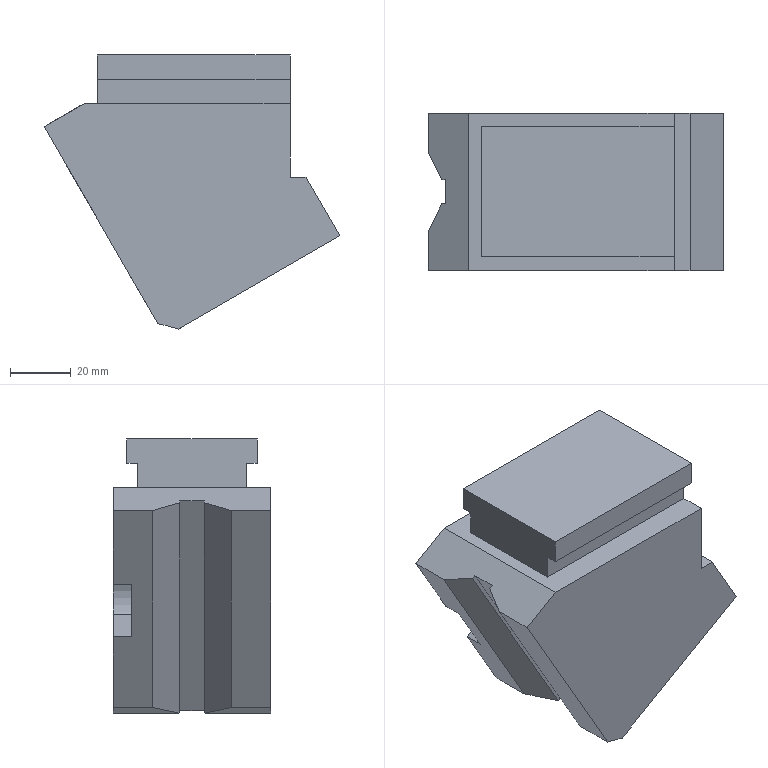Part | NX | features solid 2 | 1 solid | 33 faces | box 97.591 x 52 x 90.41 mm | volume 261017 mm3 | plane 31 | cylinder 2 | commonest cylinder face diameters 20 x2
STEP:
#1=CARTESIAN_POINT('',(-286.306,-188.,119.72));
#2=VERTEX_POINT('',#1);
#3=CARTESIAN_POINT('',(-339.567,-188.,88.97));
#4=VERTEX_POINT('',#3);
#5=CARTESIAN_POINT('',(-286.306,-188.,119.72));
#6=DIRECTION('',(-0.866,0.,-0.5));
#7=VECTOR('',#6,1000.);
#8=LINE('',#5,#7);
#9=EDGE_CURVE('',#2,#4,#8,.T.);
#10=ORIENTED_EDGE('',*,*,#9,.T.);
#11=CARTESIAN_POINT('',(-346.397,-188.,90.8));
#12=VERTEX_POINT('',#11);
#13=CARTESIAN_POINT('',(-339.567,-188.,88.97));
#14=DIRECTION('',(-0.9659,0.,0.2588));
#15=VECTOR('',#14,1000.);
#16=LINE('',#13,#15);
#17=EDGE_CURVE('',#4,#12,#16,.T.);
#18=ORIENTED_EDGE('',*,*,#17,.T.);
#19=CARTESIAN_POINT('',(-359.847,-188.,114.096));
#20=VERTEX_POINT('',#19);
#21=CARTESIAN_POINT('',(-383.897,-188.,155.752));
#22=DIRECTION('',(0.5,0.,-0.866));
#23=VECTOR('',#22,1000.);
#24=LINE('',#21,#23);
#25=EDGE_CURVE('',#20,#12,#24,.T.);
#26=ORIENTED_EDGE('',*,*,#25,.F.);
#27=CARTESIAN_POINT('',(-347.097,-188.,121.457));
#28=VERTEX_POINT('',#27);
#29=CARTESIAN_POINT('',(-329.777,-188.,131.457));
#30=DIRECTION('',(-0.866,0.,-0.5));
#31=VECTOR('',#30,1000.);
#32=LINE('',#29,#31);
#33=EDGE_CURVE('',#28,#20,#32,.T.);
#34=ORIENTED_EDGE('',*,*,#33,.F.);
#35=CARTESIAN_POINT('',(-329.777,-188.,131.457));
#36=VERTEX_POINT('',#35);
#37=CARTESIAN_POINT('',(-338.437,-188.,126.457));
#38=DIRECTION('',(0.,-1.,0.));
#39=DIRECTION('',(0.766,0.,-0.6428));
#40=AXIS2_PLACEMENT_3D('',#37,#38,#39);
#41=CIRCLE('',#40,10.);
#42=EDGE_CURVE('',#28,#36,#41,.T.);
#43=ORIENTED_EDGE('',*,*,#42,.T.);
#44=CARTESIAN_POINT('',(-339.777,-188.,148.778));
#45=VERTEX_POINT('',#44);
#46=CARTESIAN_POINT('',(-329.777,-188.,131.457));
#47=DIRECTION('',(-0.5,0.,0.866));
#48=VECTOR('',#47,1000.);
#49=LINE('',#46,#48);
#50=EDGE_CURVE('',#36,#45,#49,.T.);
#51=ORIENTED_EDGE('',*,*,#50,.T.);
#52=CARTESIAN_POINT('',(-357.097,-188.,138.778));
#53=VERTEX_POINT('',#52);
#54=CARTESIAN_POINT('',(-348.437,-188.,143.778));
#55=DIRECTION('',(0.,-1.,0.));
#56=DIRECTION('',(0.766,0.,-0.6428));
#57=AXIS2_PLACEMENT_3D('',#54,#55,#56);
#58=CIRCLE('',#57,10.);
#59=EDGE_CURVE('',#45,#53,#58,.T.);
#60=ORIENTED_EDGE('',*,*,#59,.T.);
#61=CARTESIAN_POINT('',(-369.847,-188.,131.417));
#62=VERTEX_POINT('',#61);
#63=CARTESIAN_POINT('',(-339.777,-188.,148.778));
#64=DIRECTION('',(-0.866,0.,-0.5));
#65=VECTOR('',#64,1000.);
#66=LINE('',#63,#65);
#67=EDGE_CURVE('',#53,#62,#66,.T.);
#68=ORIENTED_EDGE('',*,*,#67,.T.);
#69=CARTESIAN_POINT('',(-383.897,-188.,155.752));
#70=VERTEX_POINT('',#69);
#71=CARTESIAN_POINT('',(-383.897,-188.,155.752));
#72=DIRECTION('',(0.5,0.,-0.866));
#73=VECTOR('',#72,1000.);
#74=LINE('',#71,#73);
#75=EDGE_CURVE('',#70,#62,#74,.T.);
#76=ORIENTED_EDGE('',*,*,#75,.F.);
#77=CARTESIAN_POINT('',(-370.685,-188.,163.38));
#78=VERTEX_POINT('',#77);
#79=CARTESIAN_POINT('',(-370.685,-188.,163.38));
#80=DIRECTION('',(-0.866,0.,-0.5));
#81=VECTOR('',#80,1000.);
#82=LINE('',#79,#81);
#83=EDGE_CURVE('',#78,#70,#82,.T.);
#84=ORIENTED_EDGE('',*,*,#83,.F.);
#85=CARTESIAN_POINT('',(-302.724,-188.,163.38));
#86=VERTEX_POINT('',#85);
#87=CARTESIAN_POINT('',(-370.685,-188.,163.38));
#88=DIRECTION('',(1.,0.,0.));
#89=VECTOR('',#88,1000.);
#90=LINE('',#87,#89);
#91=EDGE_CURVE('',#78,#86,#90,.T.);
#92=ORIENTED_EDGE('',*,*,#91,.T.);
#93=CARTESIAN_POINT('',(-302.724,-188.,139.062));
#94=VERTEX_POINT('',#93);
#95=CARTESIAN_POINT('',(-302.724,-188.,155.752));
#96=DIRECTION('',(0.,0.,-1.));
#97=VECTOR('',#96,1000.);
#98=LINE('',#95,#97);
#99=EDGE_CURVE('',#86,#94,#98,.T.);
#100=ORIENTED_EDGE('',*,*,#99,.T.);
#101=CARTESIAN_POINT('',(-297.474,-188.,139.062));
#102=VERTEX_POINT('',#101);
#103=CARTESIAN_POINT('',(-383.897,-188.,139.062));
#104=DIRECTION('',(-1.,0.,0.));
#105=VECTOR('',#104,1000.);
#106=LINE('',#103,#105);
#107=EDGE_CURVE('',#102,#94,#106,.T.);
#108=ORIENTED_EDGE('',*,*,#107,.F.);
#109=CARTESIAN_POINT('',(-291.306,-188.,128.38));
#110=DIRECTION('',(0.5,0.,-0.866));
#111=VECTOR('',#110,1000.);
#112=LINE('',#109,#111);
#113=EDGE_CURVE('',#102,#2,#112,.T.);
#114=ORIENTED_EDGE('',*,*,#113,.T.);
#115=EDGE_LOOP('',(#10,#18,#26,#34,#43,#51,#60,#68,#76,#84,#92,#100,#108,#114));
#116=FACE_BOUND('',#115,.T.);
#117=CARTESIAN_POINT('',(-383.897,-188.,155.752));
#118=DIRECTION('',(0.,-1.,0.));
#119=DIRECTION('',(0.,0.,-1.));
#120=AXIS2_PLACEMENT_3D('',#117,#118,#119);
#121=PLANE('',#120);
#122=ADVANCED_FACE('',(#116),#121,.F.);
#123=ORIENTED_EDGE('',*,*,#25,.T.);
#124=CARTESIAN_POINT('',(-346.397,-201.01,90.8));
#125=VERTEX_POINT('',#124);
#126=CARTESIAN_POINT('',(-346.397,-201.01,90.8));
#127=DIRECTION('',(0.,-1.,0.));
#128=VECTOR('',#127,1000.);
#129=LINE('',#126,#128);
#130=EDGE_CURVE('',#12,#125,#129,.T.);
#131=ORIENTED_EDGE('',*,*,#130,.T.);
#132=CARTESIAN_POINT('',(-383.897,-201.01,155.752));
#133=VERTEX_POINT('',#132);
#134=CARTESIAN_POINT('',(-383.897,-201.01,155.752));
#135=DIRECTION('',(-0.5,0.,0.866));
#136=VECTOR('',#135,1000.);
#137=LINE('',#134,#136);
#138=EDGE_CURVE('',#125,#133,#137,.T.);
#139=ORIENTED_EDGE('',*,*,#138,.T.);
#140=CARTESIAN_POINT('',(-383.897,-240.,155.752));
#141=DIRECTION('',(0.,1.,0.));
#142=VECTOR('',#141,1000.);
#143=LINE('',#140,#142);
#144=EDGE_CURVE('',#133,#70,#143,.T.);
#145=ORIENTED_EDGE('',*,*,#144,.T.);
#146=ORIENTED_EDGE('',*,*,#75,.T.);
#147=CARTESIAN_POINT('',(-369.847,-194.,131.417));
#148=VERTEX_POINT('',#147);
#149=CARTESIAN_POINT('',(-369.847,-240.,131.417));
#150=DIRECTION('',(0.,1.,0.));
#151=VECTOR('',#150,1000.);
#152=LINE('',#149,#151);
#153=EDGE_CURVE('',#148,#62,#152,.T.);
#154=ORIENTED_EDGE('',*,*,#153,.F.);
#155=CARTESIAN_POINT('',(-359.847,-194.,114.096));
#156=VERTEX_POINT('',#155);
#157=CARTESIAN_POINT('',(-383.897,-194.,155.752));
#158=DIRECTION('',(-0.5,0.,0.866));
#159=VECTOR('',#158,1000.);
#160=LINE('',#157,#159);
#161=EDGE_CURVE('',#156,#148,#160,.T.);
#162=ORIENTED_EDGE('',*,*,#161,.F.);
#163=CARTESIAN_POINT('',(-359.847,-240.,114.096));
#164=DIRECTION('',(0.,1.,0.));
#165=VECTOR('',#164,1000.);
#166=LINE('',#163,#165);
#167=EDGE_CURVE('',#156,#20,#166,.T.);
#168=ORIENTED_EDGE('',*,*,#167,.T.);
#169=EDGE_LOOP('',(#123,#131,#139,#145,#146,#154,#162,#168));
#170=FACE_BOUND('',#169,.T.);
#171=CARTESIAN_POINT('',(-383.897,-240.,155.752));
#172=DIRECTION('',(0.866,0.,0.5));
#173=DIRECTION('',(0.5,0.,-0.866));
#174=AXIS2_PLACEMENT_3D('',#171,#172,#173);
#175=PLANE('',#174);
#176=ADVANCED_FACE('',(#170),#175,.F.);
#177=CARTESIAN_POINT('',(-347.097,-194.,121.457));
#178=VERTEX_POINT('',#177);
#179=CARTESIAN_POINT('',(-357.097,-194.,138.778));
#180=VERTEX_POINT('',#179);
#181=CARTESIAN_POINT('',(-347.097,-194.,121.457));
#182=DIRECTION('',(-0.5,0.,0.866));
#183=VECTOR('',#182,1000.);
#184=LINE('',#181,#183);
#185=EDGE_CURVE('',#178,#180,#184,.T.);
#186=ORIENTED_EDGE('',*,*,#185,.T.);
#187=CARTESIAN_POINT('',(-357.097,-200.,138.778));
#188=VERTEX_POINT('',#187);
#189=CARTESIAN_POINT('',(-357.097,-200.,138.778));
#190=DIRECTION('',(0.,1.,0.));
#191=VECTOR('',#190,1000.);
#192=LINE('',#189,#191);
#193=EDGE_CURVE('',#188,#180,#192,.T.);
#194=ORIENTED_EDGE('',*,*,#193,.F.);
#195=CARTESIAN_POINT('',(-347.097,-200.,121.457));
#196=VERTEX_POINT('',#195);
#197=CARTESIAN_POINT('',(-347.097,-200.,121.457));
#198=DIRECTION('',(-0.5,0.,0.866));
#199=VECTOR('',#198,1000.);
#200=LINE('',#197,#199);
#201=EDGE_CURVE('',#196,#188,#200,.T.);
#202=ORIENTED_EDGE('',*,*,#201,.F.);
#203=CARTESIAN_POINT('',(-347.097,-200.,121.457));
#204=DIRECTION('',(0.,1.,0.));
#205=VECTOR('',#204,1000.);
#206=LINE('',#203,#205);
#207=EDGE_CURVE('',#196,#178,#206,.T.);
#208=ORIENTED_EDGE('',*,*,#207,.T.);
#209=EDGE_LOOP('',(#186,#194,#202,#208));
#210=FACE_BOUND('',#209,.T.);
#211=CARTESIAN_POINT('',(-347.097,-200.,121.457));
#212=DIRECTION('',(-0.866,0.,-0.5));
#213=DIRECTION('',(-0.5,0.,0.866));
#214=AXIS2_PLACEMENT_3D('',#211,#212,#213);
#215=PLANE('',#214);
#216=ADVANCED_FACE('',(#210),#215,.F.);
#217=CARTESIAN_POINT('',(-383.897,-226.99,155.752));
#218=VERTEX_POINT('',#217);
#219=CARTESIAN_POINT('',(-346.397,-226.99,90.8));
#220=VERTEX_POINT('',#219);
#221=CARTESIAN_POINT('',(-383.897,-226.99,155.752));
#222=DIRECTION('',(0.5,0.,-0.866));
#223=VECTOR('',#222,1000.);
#224=LINE('',#221,#223);
#225=EDGE_CURVE('',#218,#220,#224,.T.);
#226=ORIENTED_EDGE('',*,*,#225,.T.);
#227=CARTESIAN_POINT('',(-346.397,-240.,90.8));
#228=VERTEX_POINT('',#227);
#229=CARTESIAN_POINT('',(-346.397,-240.,90.8));
#230=DIRECTION('',(0.,-1.,0.));
#231=VECTOR('',#230,1000.);
#232=LINE('',#229,#231);
#233=EDGE_CURVE('',#220,#228,#232,.T.);
#234=ORIENTED_EDGE('',*,*,#233,.T.);
#235=CARTESIAN_POINT('',(-383.897,-240.,155.752));
#236=VERTEX_POINT('',#235);
#237=CARTESIAN_POINT('',(-383.897,-240.,155.752));
#238=DIRECTION('',(0.5,0.,-0.866));
#239=VECTOR('',#238,1000.);
#240=LINE('',#237,#239);
#241=EDGE_CURVE('',#236,#228,#240,.T.);
#242=ORIENTED_EDGE('',*,*,#241,.F.);
#243=CARTESIAN_POINT('',(-383.897,-240.,155.752));
#244=DIRECTION('',(0.,1.,0.));
#245=VECTOR('',#244,1000.);
#246=LINE('',#243,#245);
#247=EDGE_CURVE('',#236,#218,#246,.T.);
#248=ORIENTED_EDGE('',*,*,#247,.T.);
#249=EDGE_LOOP('',(#226,#234,#242,#248));
#250=FACE_BOUND('',#249,.T.);
#251=CARTESIAN_POINT('',(-383.897,-240.,155.752));
#252=DIRECTION('',(0.866,0.,0.5));
#253=DIRECTION('',(0.5,0.,-0.866));
#254=AXIS2_PLACEMENT_3D('',#251,#252,#253);
#255=PLANE('',#254);
#256=ADVANCED_FACE('',(#250),#255,.F.);
#257=CARTESIAN_POINT('',(-378.268,-218.,159.002));
#258=VERTEX_POINT('',#257);
#259=CARTESIAN_POINT('',(-379.402,-218.,158.347));
#260=VERTEX_POINT('',#259);
#261=CARTESIAN_POINT('',(-378.268,-218.,159.002));
#262=DIRECTION('',(-0.866,0.,-0.5));
#263=VECTOR('',#262,1000.);
#264=LINE('',#261,#263);
#265=EDGE_CURVE('',#258,#260,#264,.T.);
#266=ORIENTED_EDGE('',*,*,#265,.T.);
#267=CARTESIAN_POINT('',(-383.897,-226.99,155.752));
#268=DIRECTION('',(0.433,0.866,0.25));
#269=VECTOR('',#268,1000.);
#270=LINE('',#267,#269);
#271=EDGE_CURVE('',#218,#260,#270,.T.);
#272=ORIENTED_EDGE('',*,*,#271,.F.);
#273=ORIENTED_EDGE('',*,*,#247,.F.);
#274=CARTESIAN_POINT('',(-370.685,-240.,163.38));
#275=VERTEX_POINT('',#274);
#276=CARTESIAN_POINT('',(-370.685,-240.,163.38));
#277=DIRECTION('',(-0.866,0.,-0.5));
#278=VECTOR('',#277,1000.);
#279=LINE('',#276,#278);
#280=EDGE_CURVE('',#275,#236,#279,.T.);
#281=ORIENTED_EDGE('',*,*,#280,.F.);
#282=CARTESIAN_POINT('',(-370.685,-240.,163.38));
#283=DIRECTION('',(0.,1.,0.));
#284=VECTOR('',#283,1000.);
#285=LINE('',#282,#284);
#286=EDGE_CURVE('',#275,#78,#285,.T.);
#287=ORIENTED_EDGE('',*,*,#286,.T.);
#288=ORIENTED_EDGE('',*,*,#83,.T.);
#289=ORIENTED_EDGE('',*,*,#144,.F.);
#290=CARTESIAN_POINT('',(-379.402,-210.,158.347));
#291=VERTEX_POINT('',#290);
#292=CARTESIAN_POINT('',(-383.897,-201.01,155.752));
#293=DIRECTION('',(-0.433,0.866,-0.25));
#294=VECTOR('',#293,1000.);
#295=LINE('',#292,#294);
#296=EDGE_CURVE('',#291,#133,#295,.T.);
#297=ORIENTED_EDGE('',*,*,#296,.F.);
#298=CARTESIAN_POINT('',(-378.268,-210.,159.002));
#299=VERTEX_POINT('',#298);
#300=CARTESIAN_POINT('',(-379.402,-210.,158.347));
#301=DIRECTION('',(0.866,0.,0.5));
#302=VECTOR('',#301,1000.);
#303=LINE('',#300,#302);
#304=EDGE_CURVE('',#291,#299,#303,.T.);
#305=ORIENTED_EDGE('',*,*,#304,.T.);
#306=CARTESIAN_POINT('',(-378.268,-218.,159.002));
#307=DIRECTION('',(0.,1.,0.));
#308=VECTOR('',#307,1000.);
#309=LINE('',#306,#308);
#310=EDGE_CURVE('',#258,#299,#309,.T.);
#311=ORIENTED_EDGE('',*,*,#310,.F.);
#312=EDGE_LOOP('',(#266,#272,#273,#281,#287,#288,#289,#297,#305,#311));
#313=FACE_BOUND('',#312,.T.);
#314=CARTESIAN_POINT('',(-370.685,-240.,163.38));
#315=DIRECTION('',(0.5,0.,-0.866));
#316=DIRECTION('',(-0.866,0.,-0.5));
#317=AXIS2_PLACEMENT_3D('',#314,#315,#316);
#318=PLANE('',#317);
#319=ADVANCED_FACE('',(#313),#318,.F.);
#320=CARTESIAN_POINT('',(-286.306,-240.,119.72));
#321=VERTEX_POINT('',#320);
#322=CARTESIAN_POINT('',(-339.567,-240.,88.97));
#323=VERTEX_POINT('',#322);
#324=CARTESIAN_POINT('',(-286.306,-240.,119.72));
#325=DIRECTION('',(-0.866,0.,-0.5));
#326=VECTOR('',#325,1000.);
#327=LINE('',#324,#326);
#328=EDGE_CURVE('',#321,#323,#327,.T.);
#329=ORIENTED_EDGE('',*,*,#328,.T.);
#330=CARTESIAN_POINT('',(-339.567,-218.33,88.97));
#331=VERTEX_POINT('',#330);
#332=CARTESIAN_POINT('',(-339.567,-226.99,88.97));
#333=DIRECTION('',(0.,1.,0.));
#334=VECTOR('',#333,1000.);
#335=LINE('',#332,#334);
#336=EDGE_CURVE('',#323,#331,#335,.T.);
#337=ORIENTED_EDGE('',*,*,#336,.T.);
#338=CARTESIAN_POINT('',(-339.402,-218.,89.065));
#339=VERTEX_POINT('',#338);
#340=CARTESIAN_POINT('',(-349.959,-239.115,82.97));
#341=DIRECTION('',(0.433,0.866,0.25));
#342=VECTOR('',#341,1000.);
#343=LINE('',#340,#342);
#344=EDGE_CURVE('',#331,#339,#343,.T.);
#345=ORIENTED_EDGE('',*,*,#344,.T.);
#346=CARTESIAN_POINT('',(-338.268,-218.,89.72));
#347=VERTEX_POINT('',#346);
#348=CARTESIAN_POINT('',(-338.268,-218.,89.72));
#349=DIRECTION('',(-0.866,0.,-0.5));
#350=VECTOR('',#349,1000.);
#351=LINE('',#348,#350);
#352=EDGE_CURVE('',#347,#339,#351,.T.);
#353=ORIENTED_EDGE('',*,*,#352,.F.);
#354=CARTESIAN_POINT('',(-338.268,-210.,89.72));
#355=VERTEX_POINT('',#354);
#356=CARTESIAN_POINT('',(-338.268,-218.,89.72));
#357=DIRECTION('',(0.,1.,0.));
#358=VECTOR('',#357,1000.);
#359=LINE('',#356,#358);
#360=EDGE_CURVE('',#347,#355,#359,.T.);
#361=ORIENTED_EDGE('',*,*,#360,.T.);
#362=CARTESIAN_POINT('',(-339.402,-210.,89.065));
#363=VERTEX_POINT('',#362);
#364=CARTESIAN_POINT('',(-339.402,-210.,89.065));
#365=DIRECTION('',(0.866,0.,0.5));
#366=VECTOR('',#365,1000.);
#367=LINE('',#364,#366);
#368=EDGE_CURVE('',#363,#355,#367,.T.);
#369=ORIENTED_EDGE('',*,*,#368,.F.);
#370=CARTESIAN_POINT('',(-339.567,-209.67,88.97));
#371=VERTEX_POINT('',#370);
#372=CARTESIAN_POINT('',(-339.402,-210.,89.065));
#373=DIRECTION('',(-0.433,0.866,-0.25));
#374=VECTOR('',#373,1000.);
#375=LINE('',#372,#374);
#376=EDGE_CURVE('',#363,#371,#375,.T.);
#377=ORIENTED_EDGE('',*,*,#376,.T.);
#378=CARTESIAN_POINT('',(-339.567,-188.,88.97));
#379=DIRECTION('',(0.,1.,0.));
#380=VECTOR('',#379,1000.);
#381=LINE('',#378,#380);
#382=EDGE_CURVE('',#371,#4,#381,.T.);
#383=ORIENTED_EDGE('',*,*,#382,.T.);
#384=ORIENTED_EDGE('',*,*,#9,.F.);
#385=CARTESIAN_POINT('',(-286.306,-240.,119.72));
#386=DIRECTION('',(0.,1.,0.));
#387=VECTOR('',#386,1000.);
#388=LINE('',#385,#387);
#389=EDGE_CURVE('',#321,#2,#388,.T.);
#390=ORIENTED_EDGE('',*,*,#389,.F.);
#391=EDGE_LOOP('',(#329,#337,#345,#353,#361,#369,#377,#383,#384,#390));
#392=FACE_BOUND('',#391,.T.);
#393=CARTESIAN_POINT('',(-286.306,-240.,119.72));
#394=DIRECTION('',(0.5,0.,-0.866));
#395=DIRECTION('',(-0.866,0.,-0.5));
#396=AXIS2_PLACEMENT_3D('',#393,#394,#395);
#397=PLANE('',#396);
#398=ADVANCED_FACE('',(#392),#397,.T.);
#399=ORIENTED_EDGE('',*,*,#113,.F.);
#400=CARTESIAN_POINT('',(-297.474,-240.,139.062));
#401=VERTEX_POINT('',#400);
#402=CARTESIAN_POINT('',(-297.474,-240.,139.062));
#403=DIRECTION('',(0.,1.,0.));
#404=VECTOR('',#403,1000.);
#405=LINE('',#402,#404);
#406=EDGE_CURVE('',#401,#102,#405,.T.);
#407=ORIENTED_EDGE('',*,*,#406,.F.);
#408=CARTESIAN_POINT('',(-291.306,-240.,128.38));
#409=DIRECTION('',(0.5,0.,-0.866));
#410=VECTOR('',#409,1000.);
#411=LINE('',#408,#410);
#412=EDGE_CURVE('',#401,#321,#411,.T.);
#413=ORIENTED_EDGE('',*,*,#412,.T.);
#414=ORIENTED_EDGE('',*,*,#389,.T.);
#415=EDGE_LOOP('',(#399,#407,#413,#414));
#416=FACE_BOUND('',#415,.T.);
#417=CARTESIAN_POINT('',(-291.306,-240.,128.38));
#418=DIRECTION('',(0.866,0.,0.5));
#419=DIRECTION('',(0.5,0.,-0.866));
#420=AXIS2_PLACEMENT_3D('',#417,#418,#419);
#421=PLANE('',#420);
#422=ADVANCED_FACE('',(#416),#421,.T.);
#423=CARTESIAN_POINT('',(-302.724,-196.,163.38));
#424=VERTEX_POINT('',#423);
#425=CARTESIAN_POINT('',(-302.724,-240.,163.38));
#426=DIRECTION('',(0.,-1.,0.));
#427=VECTOR('',#426,1000.);
#428=LINE('',#425,#427);
#429=EDGE_CURVE('',#86,#424,#428,.T.);
#430=ORIENTED_EDGE('',*,*,#429,.F.);
#431=ORIENTED_EDGE('',*,*,#91,.F.);
#432=ORIENTED_EDGE('',*,*,#286,.F.);
#433=CARTESIAN_POINT('',(-302.724,-240.,163.38));
#434=VERTEX_POINT('',#433);
#435=CARTESIAN_POINT('',(-370.685,-240.,163.38));
#436=DIRECTION('',(1.,0.,0.));
#437=VECTOR('',#436,1000.);
#438=LINE('',#435,#437);
#439=EDGE_CURVE('',#275,#434,#438,.T.);
#440=ORIENTED_EDGE('',*,*,#439,.T.);
#441=CARTESIAN_POINT('',(-302.724,-232.,163.38));
#442=VERTEX_POINT('',#441);
#443=CARTESIAN_POINT('',(-302.724,-240.,163.38));
#444=DIRECTION('',(0.,-1.,0.));
#445=VECTOR('',#444,1000.);
#446=LINE('',#443,#445);
#447=EDGE_CURVE('',#442,#434,#446,.T.);
#448=ORIENTED_EDGE('',*,*,#447,.F.);
#449=CARTESIAN_POINT('',(-366.306,-232.,163.38));
#450=VERTEX_POINT('',#449);
#451=CARTESIAN_POINT('',(-366.306,-232.,163.38));
#452=DIRECTION('',(1.,0.,0.));
#453=VECTOR('',#452,1000.);
#454=LINE('',#451,#453);
#455=EDGE_CURVE('',#450,#442,#454,.T.);
#456=ORIENTED_EDGE('',*,*,#455,.F.);
#457=CARTESIAN_POINT('',(-366.306,-196.,163.38));
#458=VERTEX_POINT('',#457);
#459=CARTESIAN_POINT('',(-366.306,-196.,163.38));
#460=DIRECTION('',(0.,-1.,0.));
#461=VECTOR('',#460,1000.);
#462=LINE('',#459,#461);
#463=EDGE_CURVE('',#458,#450,#462,.T.);
#464=ORIENTED_EDGE('',*,*,#463,.F.);
#465=CARTESIAN_POINT('',(-366.306,-196.,163.38));
#466=DIRECTION('',(1.,0.,0.));
#467=VECTOR('',#466,1000.);
#468=LINE('',#465,#467);
#469=EDGE_CURVE('',#458,#424,#468,.T.);
#470=ORIENTED_EDGE('',*,*,#469,.T.);
#471=EDGE_LOOP('',(#430,#431,#432,#440,#448,#456,#464,#470));
#472=FACE_BOUND('',#471,.T.);
#473=CARTESIAN_POINT('',(-370.685,-240.,163.38));
#474=DIRECTION('',(0.,0.,1.));
#475=DIRECTION('',(1.,0.,0.));
#476=AXIS2_PLACEMENT_3D('',#473,#474,#475);
#477=PLANE('',#476);
#478=ADVANCED_FACE('',(#472),#477,.T.);
#479=ORIENTED_EDGE('',*,*,#241,.T.);
#480=CARTESIAN_POINT('',(-397.623,-240.,104.526));
#481=DIRECTION('',(0.9659,0.,-0.2588));
#482=VECTOR('',#481,1000.);
#483=LINE('',#480,#482);
#484=EDGE_CURVE('',#228,#323,#483,.T.);
#485=ORIENTED_EDGE('',*,*,#484,.T.);
#486=ORIENTED_EDGE('',*,*,#328,.F.);
#487=ORIENTED_EDGE('',*,*,#412,.F.);
#488=CARTESIAN_POINT('',(-302.724,-240.,139.062));
#489=VERTEX_POINT('',#488);
#490=CARTESIAN_POINT('',(-302.724,-240.,139.062));
#491=DIRECTION('',(1.,0.,0.));
#492=VECTOR('',#491,1000.);
#493=LINE('',#490,#492);
#494=EDGE_CURVE('',#489,#401,#493,.T.);
#495=ORIENTED_EDGE('',*,*,#494,.F.);
#496=CARTESIAN_POINT('',(-302.724,-240.,139.062));
#497=DIRECTION('',(0.,0.,1.));
#498=VECTOR('',#497,1000.);
#499=LINE('',#496,#498);
#500=EDGE_CURVE('',#489,#434,#499,.T.);
#501=ORIENTED_EDGE('',*,*,#500,.T.);
#502=ORIENTED_EDGE('',*,*,#439,.F.);
#503=ORIENTED_EDGE('',*,*,#280,.T.);
#504=EDGE_LOOP('',(#479,#485,#486,#487,#495,#501,#502,#503));
#505=FACE_BOUND('',#504,.T.);
#506=CARTESIAN_POINT('',(-383.897,-240.,155.752));
#507=DIRECTION('',(0.,-1.,0.));
#508=DIRECTION('',(0.,0.,-1.));
#509=AXIS2_PLACEMENT_3D('',#506,#507,#508);
#510=PLANE('',#509);
#511=ADVANCED_FACE('',(#505),#510,.T.);
#512=CARTESIAN_POINT('',(-366.306,-232.,171.38));
#513=VERTEX_POINT('',#512);
#514=CARTESIAN_POINT('',(-366.306,-232.,171.38));
#515=DIRECTION('',(0.,0.,-1.));
#516=VECTOR('',#515,1000.);
#517=LINE('',#514,#516);
#518=EDGE_CURVE('',#513,#450,#517,.T.);
#519=ORIENTED_EDGE('',*,*,#518,.F.);
#520=CARTESIAN_POINT('',(-366.306,-235.5,171.38));
#521=VERTEX_POINT('',#520);
#522=CARTESIAN_POINT('',(-366.306,-192.5,171.38));
#523=DIRECTION('',(0.,-1.,0.));
#524=VECTOR('',#523,1000.);
#525=LINE('',#522,#524);
#526=EDGE_CURVE('',#513,#521,#525,.T.);
#527=ORIENTED_EDGE('',*,*,#526,.T.);
#528=CARTESIAN_POINT('',(-366.306,-235.5,179.38));
#529=VERTEX_POINT('',#528);
#530=CARTESIAN_POINT('',(-366.306,-235.5,179.38));
#531=DIRECTION('',(0.,0.,-1.));
#532=VECTOR('',#531,1000.);
#533=LINE('',#530,#532);
#534=EDGE_CURVE('',#529,#521,#533,.T.);
#535=ORIENTED_EDGE('',*,*,#534,.F.);
#536=CARTESIAN_POINT('',(-366.306,-192.5,179.38));
#537=VERTEX_POINT('',#536);
#538=CARTESIAN_POINT('',(-366.306,-192.5,179.38));
#539=DIRECTION('',(0.,-1.,0.));
#540=VECTOR('',#539,1000.);
#541=LINE('',#538,#540);
#542=EDGE_CURVE('',#537,#529,#541,.T.);
#543=ORIENTED_EDGE('',*,*,#542,.F.);
#544=CARTESIAN_POINT('',(-366.306,-192.5,171.38));
#545=VERTEX_POINT('',#544);
#546=CARTESIAN_POINT('',(-366.306,-192.5,179.38));
#547=DIRECTION('',(0.,0.,-1.));
#548=VECTOR('',#547,1000.);
#549=LINE('',#546,#548);
#550=EDGE_CURVE('',#537,#545,#549,.T.);
#551=ORIENTED_EDGE('',*,*,#550,.T.);
#552=CARTESIAN_POINT('',(-366.306,-196.,171.38));
#553=VERTEX_POINT('',#552);
#554=CARTESIAN_POINT('',(-366.306,-192.5,171.38));
#555=DIRECTION('',(0.,-1.,0.));
#556=VECTOR('',#555,1000.);
#557=LINE('',#554,#556);
#558=EDGE_CURVE('',#545,#553,#557,.T.);
#559=ORIENTED_EDGE('',*,*,#558,.T.);
#560=CARTESIAN_POINT('',(-366.306,-196.,171.38));
#561=DIRECTION('',(0.,0.,-1.));
#562=VECTOR('',#561,1000.);
#563=LINE('',#560,#562);
#564=EDGE_CURVE('',#553,#458,#563,.T.);
#565=ORIENTED_EDGE('',*,*,#564,.T.);
#566=ORIENTED_EDGE('',*,*,#463,.T.);
#567=EDGE_LOOP('',(#519,#527,#535,#543,#551,#559,#565,#566));
#568=FACE_BOUND('',#567,.T.);
#569=CARTESIAN_POINT('',(-366.306,-196.,171.38));
#570=DIRECTION('',(-1.,0.,0.));
#571=DIRECTION('',(0.,0.,1.));
#572=AXIS2_PLACEMENT_3D('',#569,#570,#571);
#573=PLANE('',#572);
#574=ADVANCED_FACE('',(#568),#573,.T.);
#575=CARTESIAN_POINT('',(-302.724,-196.,171.38));
#576=VERTEX_POINT('',#575);
#577=CARTESIAN_POINT('',(-291.306,-196.,171.38));
#578=DIRECTION('',(-1.,0.,0.));
#579=VECTOR('',#578,1000.);
#580=LINE('',#577,#579);
#581=EDGE_CURVE('',#576,#553,#580,.T.);
#582=ORIENTED_EDGE('',*,*,#581,.F.);
#583=CARTESIAN_POINT('',(-302.724,-196.,171.38));
#584=DIRECTION('',(0.,0.,-1.));
#585=VECTOR('',#584,1000.);
#586=LINE('',#583,#585);
#587=EDGE_CURVE('',#576,#424,#586,.T.);
#588=ORIENTED_EDGE('',*,*,#587,.T.);
#589=ORIENTED_EDGE('',*,*,#469,.F.);
#590=ORIENTED_EDGE('',*,*,#564,.F.);
#591=EDGE_LOOP('',(#582,#588,#589,#590));
#592=FACE_BOUND('',#591,.T.);
#593=CARTESIAN_POINT('',(-291.306,-196.,171.38));
#594=DIRECTION('',(0.,-1.,0.));
#595=DIRECTION('',(0.,0.,-1.));
#596=AXIS2_PLACEMENT_3D('',#593,#594,#595);
#597=PLANE('',#596);
#598=ADVANCED_FACE('',(#592),#597,.F.);
#599=CARTESIAN_POINT('',(-302.724,-232.,171.38));
#600=VERTEX_POINT('',#599);
#601=CARTESIAN_POINT('',(-302.724,-232.,171.38));
#602=DIRECTION('',(0.,0.,-1.));
#603=VECTOR('',#602,1000.);
#604=LINE('',#601,#603);
#605=EDGE_CURVE('',#600,#442,#604,.T.);
#606=ORIENTED_EDGE('',*,*,#605,.F.);
#607=CARTESIAN_POINT('',(-291.306,-232.,171.38));
#608=DIRECTION('',(-1.,0.,0.));
#609=VECTOR('',#608,1000.);
#610=LINE('',#607,#609);
#611=EDGE_CURVE('',#600,#513,#610,.T.);
#612=ORIENTED_EDGE('',*,*,#611,.T.);
#613=ORIENTED_EDGE('',*,*,#518,.T.);
#614=ORIENTED_EDGE('',*,*,#455,.T.);
#615=EDGE_LOOP('',(#606,#612,#613,#614));
#616=FACE_BOUND('',#615,.T.);
#617=CARTESIAN_POINT('',(-291.306,-232.,171.38));
#618=DIRECTION('',(0.,-1.,0.));
#619=DIRECTION('',(0.,0.,-1.));
#620=AXIS2_PLACEMENT_3D('',#617,#618,#619);
#621=PLANE('',#620);
#622=ADVANCED_FACE('',(#616),#621,.T.);
#623=CARTESIAN_POINT('',(-302.724,-192.5,171.38));
#624=VERTEX_POINT('',#623);
#625=CARTESIAN_POINT('',(-291.306,-192.5,171.38));
#626=DIRECTION('',(-1.,0.,0.));
#627=VECTOR('',#626,1000.);
#628=LINE('',#625,#627);
#629=EDGE_CURVE('',#624,#545,#628,.T.);
#630=ORIENTED_EDGE('',*,*,#629,.F.);
#631=CARTESIAN_POINT('',(-302.724,-192.5,171.38));
#632=DIRECTION('',(0.,-1.,0.));
#633=VECTOR('',#632,1000.);
#634=LINE('',#631,#633);
#635=EDGE_CURVE('',#624,#576,#634,.T.);
#636=ORIENTED_EDGE('',*,*,#635,.T.);
#637=ORIENTED_EDGE('',*,*,#581,.T.);
#638=ORIENTED_EDGE('',*,*,#558,.F.);
#639=EDGE_LOOP('',(#630,#636,#637,#638));
#640=FACE_BOUND('',#639,.T.);
#641=CARTESIAN_POINT('',(-291.306,-192.5,171.38));
#642=DIRECTION('',(0.,0.,1.));
#643=DIRECTION('',(1.,0.,0.));
#644=AXIS2_PLACEMENT_3D('',#641,#642,#643);
#645=PLANE('',#644);
#646=ADVANCED_FACE('',(#640),#645,.F.);
#647=ORIENTED_EDGE('',*,*,#611,.F.);
#648=CARTESIAN_POINT('',(-302.724,-235.5,171.38));
#649=VERTEX_POINT('',#648);
#650=CARTESIAN_POINT('',(-302.724,-192.5,171.38));
#651=DIRECTION('',(0.,-1.,0.));
#652=VECTOR('',#651,1000.);
#653=LINE('',#650,#652);
#654=EDGE_CURVE('',#600,#649,#653,.T.);
#655=ORIENTED_EDGE('',*,*,#654,.T.);
#656=CARTESIAN_POINT('',(-291.306,-235.5,171.38));
#657=DIRECTION('',(-1.,0.,0.));
#658=VECTOR('',#657,1000.);
#659=LINE('',#656,#658);
#660=EDGE_CURVE('',#649,#521,#659,.T.);
#661=ORIENTED_EDGE('',*,*,#660,.T.);
#662=ORIENTED_EDGE('',*,*,#526,.F.);
#663=EDGE_LOOP('',(#647,#655,#661,#662));
#664=FACE_BOUND('',#663,.T.);
#665=CARTESIAN_POINT('',(-291.306,-192.5,171.38));
#666=DIRECTION('',(0.,0.,1.));
#667=DIRECTION('',(1.,0.,0.));
#668=AXIS2_PLACEMENT_3D('',#665,#666,#667);
#669=PLANE('',#668);
#670=ADVANCED_FACE('',(#664),#669,.F.);
#671=CARTESIAN_POINT('',(-302.724,-235.5,179.38));
#672=VERTEX_POINT('',#671);
#673=CARTESIAN_POINT('',(-366.306,-235.5,179.38));
#674=DIRECTION('',(1.,0.,0.));
#675=VECTOR('',#674,1000.);
#676=LINE('',#673,#675);
#677=EDGE_CURVE('',#529,#672,#676,.T.);
#678=ORIENTED_EDGE('',*,*,#677,.T.);
#679=CARTESIAN_POINT('',(-302.724,-192.5,179.38));
#680=VERTEX_POINT('',#679);
#681=CARTESIAN_POINT('',(-302.724,-192.5,179.38));
#682=DIRECTION('',(0.,1.,0.));
#683=VECTOR('',#682,1000.);
#684=LINE('',#681,#683);
#685=EDGE_CURVE('',#672,#680,#684,.T.);
#686=ORIENTED_EDGE('',*,*,#685,.T.);
#687=CARTESIAN_POINT('',(-366.306,-192.5,179.38));
#688=DIRECTION('',(1.,0.,0.));
#689=VECTOR('',#688,1000.);
#690=LINE('',#687,#689);
#691=EDGE_CURVE('',#537,#680,#690,.T.);
#692=ORIENTED_EDGE('',*,*,#691,.F.);
#693=ORIENTED_EDGE('',*,*,#542,.T.);
#694=EDGE_LOOP('',(#678,#686,#692,#693));
#695=FACE_BOUND('',#694,.T.);
#696=CARTESIAN_POINT('',(-366.306,-192.5,179.38));
#697=DIRECTION('',(0.,0.,-1.));
#698=DIRECTION('',(-1.,0.,0.));
#699=AXIS2_PLACEMENT_3D('',#696,#697,#698);
#700=PLANE('',#699);
#701=ADVANCED_FACE('',(#695),#700,.F.);
#702=ORIENTED_EDGE('',*,*,#691,.T.);
#703=CARTESIAN_POINT('',(-302.724,-192.5,171.38));
#704=DIRECTION('',(0.,0.,-1.));
#705=VECTOR('',#704,1000.);
#706=LINE('',#703,#705);
#707=EDGE_CURVE('',#680,#624,#706,.T.);
#708=ORIENTED_EDGE('',*,*,#707,.T.);
#709=ORIENTED_EDGE('',*,*,#629,.T.);
#710=ORIENTED_EDGE('',*,*,#550,.F.);
#711=EDGE_LOOP('',(#702,#708,#709,#710));
#712=FACE_BOUND('',#711,.T.);
#713=CARTESIAN_POINT('',(-366.306,-192.5,171.38));
#714=DIRECTION('',(0.,-1.,0.));
#715=DIRECTION('',(0.,0.,-1.));
#716=AXIS2_PLACEMENT_3D('',#713,#714,#715);
#717=PLANE('',#716);
#718=ADVANCED_FACE('',(#712),#717,.F.);
#719=CARTESIAN_POINT('',(-302.724,-235.5,171.38));
#720=DIRECTION('',(0.,0.,-1.));
#721=VECTOR('',#720,1000.);
#722=LINE('',#719,#721);
#723=EDGE_CURVE('',#672,#649,#722,.T.);
#724=ORIENTED_EDGE('',*,*,#723,.F.);
#725=ORIENTED_EDGE('',*,*,#677,.F.);
#726=ORIENTED_EDGE('',*,*,#534,.T.);
#727=ORIENTED_EDGE('',*,*,#660,.F.);
#728=EDGE_LOOP('',(#724,#725,#726,#727));
#729=FACE_BOUND('',#728,.T.);
#730=CARTESIAN_POINT('',(-366.306,-235.5,171.38));
#731=DIRECTION('',(0.,-1.,0.));
#732=DIRECTION('',(0.,0.,-1.));
#733=AXIS2_PLACEMENT_3D('',#730,#731,#732);
#734=PLANE('',#733);
#735=ADVANCED_FACE('',(#729),#734,.T.);
#736=ORIENTED_EDGE('',*,*,#406,.T.);
#737=ORIENTED_EDGE('',*,*,#107,.T.);
#738=CARTESIAN_POINT('',(-302.724,-240.,139.062));
#739=DIRECTION('',(0.,1.,0.));
#740=VECTOR('',#739,1000.);
#741=LINE('',#738,#740);
#742=EDGE_CURVE('',#489,#94,#741,.T.);
#743=ORIENTED_EDGE('',*,*,#742,.F.);
#744=ORIENTED_EDGE('',*,*,#494,.T.);
#745=EDGE_LOOP('',(#736,#737,#743,#744));
#746=FACE_BOUND('',#745,.T.);
#747=CARTESIAN_POINT('',(-302.724,-240.,139.062));
#748=DIRECTION('',(0.,0.,1.));
#749=DIRECTION('',(1.,0.,0.));
#750=AXIS2_PLACEMENT_3D('',#747,#748,#749);
#751=PLANE('',#750);
#752=ADVANCED_FACE('',(#746),#751,.T.);
#753=ORIENTED_EDGE('',*,*,#99,.F.);
#754=ORIENTED_EDGE('',*,*,#429,.T.);
#755=ORIENTED_EDGE('',*,*,#587,.F.);
#756=ORIENTED_EDGE('',*,*,#635,.F.);
#757=ORIENTED_EDGE('',*,*,#707,.F.);
#758=ORIENTED_EDGE('',*,*,#685,.F.);
#759=ORIENTED_EDGE('',*,*,#723,.T.);
#760=ORIENTED_EDGE('',*,*,#654,.F.);
#761=ORIENTED_EDGE('',*,*,#605,.T.);
#762=ORIENTED_EDGE('',*,*,#447,.T.);
#763=ORIENTED_EDGE('',*,*,#500,.F.);
#764=ORIENTED_EDGE('',*,*,#742,.T.);
#765=EDGE_LOOP('',(#753,#754,#755,#756,#757,#758,#759,#760,#761,#762,#763,#764));
#766=FACE_BOUND('',#765,.T.);
#767=CARTESIAN_POINT('',(-302.724,-240.,139.062));
#768=DIRECTION('',(-1.,0.,0.));
#769=DIRECTION('',(0.,0.,1.));
#770=AXIS2_PLACEMENT_3D('',#767,#768,#769);
#771=PLANE('',#770);
#772=ADVANCED_FACE('',(#766),#771,.F.);
#773=ORIENTED_EDGE('',*,*,#344,.F.);
#774=CARTESIAN_POINT('',(-349.821,-231.332,91.718));
#775=DIRECTION('',(-0.6109,-0.7746,0.1637));
#776=VECTOR('',#775,1000.);
#777=LINE('',#774,#776);
#778=EDGE_CURVE('',#331,#220,#777,.T.);
#779=ORIENTED_EDGE('',*,*,#778,.T.);
#780=ORIENTED_EDGE('',*,*,#225,.F.);
#781=ORIENTED_EDGE('',*,*,#271,.T.);
#782=CARTESIAN_POINT('',(-339.402,-218.,89.065));
#783=DIRECTION('',(-0.5,0.,0.866));
#784=VECTOR('',#783,1000.);
#785=LINE('',#782,#784);
#786=EDGE_CURVE('',#339,#260,#785,.T.);
#787=ORIENTED_EDGE('',*,*,#786,.F.);
#788=EDGE_LOOP('',(#773,#779,#780,#781,#787));
#789=FACE_BOUND('',#788,.T.);
#790=CARTESIAN_POINT('',(-343.897,-226.99,86.47));
#791=DIRECTION('',(0.75,-0.5,0.433));
#792=DIRECTION('',(0.5547,0.8321,0.));
#793=AXIS2_PLACEMENT_3D('',#790,#791,#792);
#794=PLANE('',#793);
#795=ADVANCED_FACE('',(#789),#794,.F.);
#796=ORIENTED_EDGE('',*,*,#138,.F.);
#797=CARTESIAN_POINT('',(-325.215,-227.868,85.124));
#798=DIRECTION('',(0.6109,-0.7746,-0.1637));
#799=VECTOR('',#798,1000.);
#800=LINE('',#797,#799);
#801=EDGE_CURVE('',#125,#371,#800,.T.);
#802=ORIENTED_EDGE('',*,*,#801,.T.);
#803=ORIENTED_EDGE('',*,*,#376,.F.);
#804=CARTESIAN_POINT('',(-339.402,-210.,89.065));
#805=DIRECTION('',(-0.5,0.,0.866));
#806=VECTOR('',#805,1000.);
#807=LINE('',#804,#806);
#808=EDGE_CURVE('',#363,#291,#807,.T.);
#809=ORIENTED_EDGE('',*,*,#808,.T.);
#810=ORIENTED_EDGE('',*,*,#296,.T.);
#811=EDGE_LOOP('',(#796,#802,#803,#809,#810));
#812=FACE_BOUND('',#811,.T.);
#813=CARTESIAN_POINT('',(-343.897,-201.01,86.47));
#814=DIRECTION('',(0.75,0.5,0.433));
#815=DIRECTION('',(-0.5547,0.8321,0.));
#816=AXIS2_PLACEMENT_3D('',#813,#814,#815);
#817=PLANE('',#816);
#818=ADVANCED_FACE('',(#812),#817,.F.);
#819=ORIENTED_EDGE('',*,*,#310,.T.);
#820=CARTESIAN_POINT('',(-338.268,-210.,89.72));
#821=DIRECTION('',(-0.5,0.,0.866));
#822=VECTOR('',#821,1000.);
#823=LINE('',#820,#822);
#824=EDGE_CURVE('',#355,#299,#823,.T.);
#825=ORIENTED_EDGE('',*,*,#824,.F.);
#826=ORIENTED_EDGE('',*,*,#360,.F.);
#827=CARTESIAN_POINT('',(-338.268,-218.,89.72));
#828=DIRECTION('',(-0.5,0.,0.866));
#829=VECTOR('',#828,1000.);
#830=LINE('',#827,#829);
#831=EDGE_CURVE('',#347,#258,#830,.T.);
#832=ORIENTED_EDGE('',*,*,#831,.T.);
#833=EDGE_LOOP('',(#819,#825,#826,#832));
#834=FACE_BOUND('',#833,.T.);
#835=CARTESIAN_POINT('',(-338.268,-218.,89.72));
#836=DIRECTION('',(0.866,0.,0.5));
#837=DIRECTION('',(0.5,0.,-0.866));
#838=AXIS2_PLACEMENT_3D('',#835,#836,#837);
#839=PLANE('',#838);
#840=ADVANCED_FACE('',(#834),#839,.F.);
#841=ORIENTED_EDGE('',*,*,#304,.F.);
#842=ORIENTED_EDGE('',*,*,#808,.F.);
#843=ORIENTED_EDGE('',*,*,#368,.T.);
#844=ORIENTED_EDGE('',*,*,#824,.T.);
#845=EDGE_LOOP('',(#841,#842,#843,#844));
#846=FACE_BOUND('',#845,.T.);
#847=CARTESIAN_POINT('',(-339.402,-210.,89.065));
#848=DIRECTION('',(0.,-1.,0.));
#849=DIRECTION('',(1.,0.,0.));
#850=AXIS2_PLACEMENT_3D('',#847,#848,#849);
#851=PLANE('',#850);
#852=ADVANCED_FACE('',(#846),#851,.T.);
#853=ORIENTED_EDGE('',*,*,#265,.F.);
#854=ORIENTED_EDGE('',*,*,#831,.F.);
#855=ORIENTED_EDGE('',*,*,#352,.T.);
#856=ORIENTED_EDGE('',*,*,#786,.T.);
#857=EDGE_LOOP('',(#853,#854,#855,#856));
#858=FACE_BOUND('',#857,.T.);
#859=CARTESIAN_POINT('',(-338.268,-218.,89.72));
#860=DIRECTION('',(0.,1.,0.));
#861=DIRECTION('',(-1.,0.,0.));
#862=AXIS2_PLACEMENT_3D('',#859,#860,#861);
#863=PLANE('',#862);
#864=ADVANCED_FACE('',(#858),#863,.T.);
#865=ORIENTED_EDGE('',*,*,#42,.F.);
#866=CARTESIAN_POINT('',(-347.097,-200.,121.457));
#867=DIRECTION('',(0.,-1.,0.));
#868=VECTOR('',#867,1000.);
#869=LINE('',#866,#868);
#870=EDGE_CURVE('',#28,#178,#869,.T.);
#871=ORIENTED_EDGE('',*,*,#870,.T.);
#872=ORIENTED_EDGE('',*,*,#207,.F.);
#873=CARTESIAN_POINT('',(-329.777,-200.,131.457));
#874=VERTEX_POINT('',#873);
#875=CARTESIAN_POINT('',(-338.437,-200.,126.457));
#876=DIRECTION('',(0.,-1.,0.));
#877=DIRECTION('',(0.766,0.,-0.6428));
#878=AXIS2_PLACEMENT_3D('',#875,#876,#877);
#879=CIRCLE('',#878,10.);
#880=EDGE_CURVE('',#196,#874,#879,.T.);
#881=ORIENTED_EDGE('',*,*,#880,.T.);
#882=CARTESIAN_POINT('',(-329.777,-200.,131.457));
#883=DIRECTION('',(0.,1.,0.));
#884=VECTOR('',#883,1000.);
#885=LINE('',#882,#884);
#886=EDGE_CURVE('',#874,#36,#885,.T.);
#887=ORIENTED_EDGE('',*,*,#886,.T.);
#888=EDGE_LOOP('',(#865,#871,#872,#881,#887));
#889=FACE_BOUND('',#888,.T.);
#890=CARTESIAN_POINT('',(-338.437,-200.,126.457));
#891=DIRECTION('',(0.,1.,0.));
#892=DIRECTION('',(0.,0.,1.));
#893=AXIS2_PLACEMENT_3D('',#890,#891,#892);
#894=CYLINDRICAL_SURFACE('',#893,10.);
#895=ADVANCED_FACE('',(#889),#894,.F.);
#896=ORIENTED_EDGE('',*,*,#50,.F.);
#897=ORIENTED_EDGE('',*,*,#886,.F.);
#898=CARTESIAN_POINT('',(-339.777,-200.,148.778));
#899=VERTEX_POINT('',#898);
#900=CARTESIAN_POINT('',(-329.777,-200.,131.457));
#901=DIRECTION('',(-0.5,0.,0.866));
#902=VECTOR('',#901,1000.);
#903=LINE('',#900,#902);
#904=EDGE_CURVE('',#874,#899,#903,.T.);
#905=ORIENTED_EDGE('',*,*,#904,.T.);
#906=CARTESIAN_POINT('',(-339.777,-200.,148.778));
#907=DIRECTION('',(0.,1.,0.));
#908=VECTOR('',#907,1000.);
#909=LINE('',#906,#908);
#910=EDGE_CURVE('',#899,#45,#909,.T.);
#911=ORIENTED_EDGE('',*,*,#910,.T.);
#912=EDGE_LOOP('',(#896,#897,#905,#911));
#913=FACE_BOUND('',#912,.T.);
#914=CARTESIAN_POINT('',(-329.777,-200.,131.457));
#915=DIRECTION('',(-0.866,0.,-0.5));
#916=DIRECTION('',(-0.5,0.,0.866));
#917=AXIS2_PLACEMENT_3D('',#914,#915,#916);
#918=PLANE('',#917);
#919=ADVANCED_FACE('',(#913),#918,.T.);
#920=ORIENTED_EDGE('',*,*,#59,.F.);
#921=ORIENTED_EDGE('',*,*,#910,.F.);
#922=CARTESIAN_POINT('',(-348.437,-200.,143.778));
#923=DIRECTION('',(0.,-1.,0.));
#924=DIRECTION('',(0.766,0.,-0.6428));
#925=AXIS2_PLACEMENT_3D('',#922,#923,#924);
#926=CIRCLE('',#925,10.);
#927=EDGE_CURVE('',#899,#188,#926,.T.);
#928=ORIENTED_EDGE('',*,*,#927,.T.);
#929=ORIENTED_EDGE('',*,*,#193,.T.);
#930=CARTESIAN_POINT('',(-357.097,-200.,138.778));
#931=DIRECTION('',(0.,-1.,0.));
#932=VECTOR('',#931,1000.);
#933=LINE('',#930,#932);
#934=EDGE_CURVE('',#53,#180,#933,.T.);
#935=ORIENTED_EDGE('',*,*,#934,.F.);
#936=EDGE_LOOP('',(#920,#921,#928,#929,#935));
#937=FACE_BOUND('',#936,.T.);
#938=CARTESIAN_POINT('',(-348.437,-200.,143.778));
#939=DIRECTION('',(0.,1.,0.));
#940=DIRECTION('',(0.,0.,1.));
#941=AXIS2_PLACEMENT_3D('',#938,#939,#940);
#942=CYLINDRICAL_SURFACE('',#941,10.);
#943=ADVANCED_FACE('',(#937),#942,.F.);
#944=ORIENTED_EDGE('',*,*,#880,.F.);
#945=ORIENTED_EDGE('',*,*,#201,.T.);
#946=ORIENTED_EDGE('',*,*,#927,.F.);
#947=ORIENTED_EDGE('',*,*,#904,.F.);
#948=EDGE_LOOP('',(#944,#945,#946,#947));
#949=FACE_BOUND('',#948,.T.);
#950=CARTESIAN_POINT('',(-338.437,-200.,126.457));
#951=DIRECTION('',(0.,-1.,0.));
#952=DIRECTION('',(0.,0.,-1.));
#953=AXIS2_PLACEMENT_3D('',#950,#951,#952);
#954=PLANE('',#953);
#955=ADVANCED_FACE('',(#949),#954,.F.);
#956=ORIENTED_EDGE('',*,*,#161,.T.);
#957=CARTESIAN_POINT('',(-377.016,-194.,127.278));
#958=DIRECTION('',(0.866,0.,0.5));
#959=VECTOR('',#958,1000.);
#960=LINE('',#957,#959);
#961=EDGE_CURVE('',#148,#180,#960,.T.);
#962=ORIENTED_EDGE('',*,*,#961,.T.);
#963=ORIENTED_EDGE('',*,*,#185,.F.);
#964=CARTESIAN_POINT('',(-367.016,-194.,109.957));
#965=DIRECTION('',(0.866,0.,0.5));
#966=VECTOR('',#965,1000.);
#967=LINE('',#964,#966);
#968=EDGE_CURVE('',#156,#178,#967,.T.);
#969=ORIENTED_EDGE('',*,*,#968,.F.);
#970=EDGE_LOOP('',(#956,#962,#963,#969));
#971=FACE_BOUND('',#970,.T.);
#972=CARTESIAN_POINT('',(-377.016,-194.,127.278));
#973=DIRECTION('',(0.,1.,0.));
#974=DIRECTION('',(0.6428,0.,0.766));
#975=AXIS2_PLACEMENT_3D('',#972,#973,#974);
#976=PLANE('',#975);
#977=ADVANCED_FACE('',(#971),#976,.T.);
#978=ORIENTED_EDGE('',*,*,#153,.T.);
#979=ORIENTED_EDGE('',*,*,#67,.F.);
#980=ORIENTED_EDGE('',*,*,#934,.T.);
#981=ORIENTED_EDGE('',*,*,#961,.F.);
#982=EDGE_LOOP('',(#978,#979,#980,#981));
#983=FACE_BOUND('',#982,.T.);
#984=CARTESIAN_POINT('',(-339.777,-194.,148.778));
#985=DIRECTION('',(0.5,0.,-0.866));
#986=DIRECTION('',(0.866,0.,0.5));
#987=AXIS2_PLACEMENT_3D('',#984,#985,#986);
#988=PLANE('',#987);
#989=ADVANCED_FACE('',(#983),#988,.T.);
#990=ORIENTED_EDGE('',*,*,#968,.T.);
#991=ORIENTED_EDGE('',*,*,#870,.F.);
#992=ORIENTED_EDGE('',*,*,#33,.T.);
#993=ORIENTED_EDGE('',*,*,#167,.F.);
#994=EDGE_LOOP('',(#990,#991,#992,#993));
#995=FACE_BOUND('',#994,.T.);
#996=CARTESIAN_POINT('',(-329.777,-194.,131.457));
#997=DIRECTION('',(0.5,0.,-0.866));
#998=DIRECTION('',(0.866,0.,0.5));
#999=AXIS2_PLACEMENT_3D('',#996,#997,#998);
#1000=PLANE('',#999);
#1001=ADVANCED_FACE('',(#995),#1000,.F.);
#1002=ORIENTED_EDGE('',*,*,#801,.F.);
#1003=ORIENTED_EDGE('',*,*,#130,.F.);
#1004=ORIENTED_EDGE('',*,*,#17,.F.);
#1005=ORIENTED_EDGE('',*,*,#382,.F.);
#1006=EDGE_LOOP('',(#1002,#1003,#1004,#1005));
#1007=FACE_BOUND('',#1006,.T.);
#1008=CARTESIAN_POINT('',(-339.567,-240.,88.97));
#1009=DIRECTION('',(-0.2588,0.,-0.9659));
#1010=DIRECTION('',(-0.9659,0.,0.2588));
#1011=AXIS2_PLACEMENT_3D('',#1008,#1009,#1010);
#1012=PLANE('',#1011);
#1013=ADVANCED_FACE('',(#1007),#1012,.T.);
#1014=ORIENTED_EDGE('',*,*,#484,.F.);
#1015=ORIENTED_EDGE('',*,*,#233,.F.);
#1016=ORIENTED_EDGE('',*,*,#778,.F.);
#1017=ORIENTED_EDGE('',*,*,#336,.F.);
#1018=EDGE_LOOP('',(#1014,#1015,#1016,#1017));
#1019=FACE_BOUND('',#1018,.T.);
#1020=CARTESIAN_POINT('',(-339.567,-240.,88.97));
#1021=DIRECTION('',(-0.2588,0.,-0.9659));
#1022=DIRECTION('',(-0.9659,0.,0.2588));
#1023=AXIS2_PLACEMENT_3D('',#1020,#1021,#1022);
#1024=PLANE('',#1023);
#1025=ADVANCED_FACE('',(#1019),#1024,.T.);
#1026=CLOSED_SHELL('',(#122,#176,#216,#256,#319,#398,#422,#478,#511,#574,#598,#622,#646,#670,#701,#718,#735,#752,#772,#795,#818,#840,#852,#864,#895,#919,#943,#955,#977,#989,#1001,#1013,#1025));
#1027=MANIFOLD_SOLID_BREP('',#1026);
#1028=(LENGTH_UNIT()NAMED_UNIT(*)SI_UNIT(.MILLI.,.METRE.));
#1029=UNCERTAINTY_MEASURE_WITH_UNIT(LENGTH_MEASURE(0.00001),#1028,'','');
#1030=(NAMED_UNIT(*)PLANE_ANGLE_UNIT()SI_UNIT($,.RADIAN.));
#1031=(NAMED_UNIT(*)SI_UNIT($,.STERADIAN.)SOLID_ANGLE_UNIT());
#1032=(GEOMETRIC_REPRESENTATION_CONTEXT(3)GLOBAL_UNCERTAINTY_ASSIGNED_CONTEXT((#1029))GLOBAL_UNIT_ASSIGNED_CONTEXT((#1028,#1030,#1031))REPRESENTATION_CONTEXT('',''));
#1033=ADVANCED_BREP_SHAPE_REPRESENTATION('',(#1027),#1032);